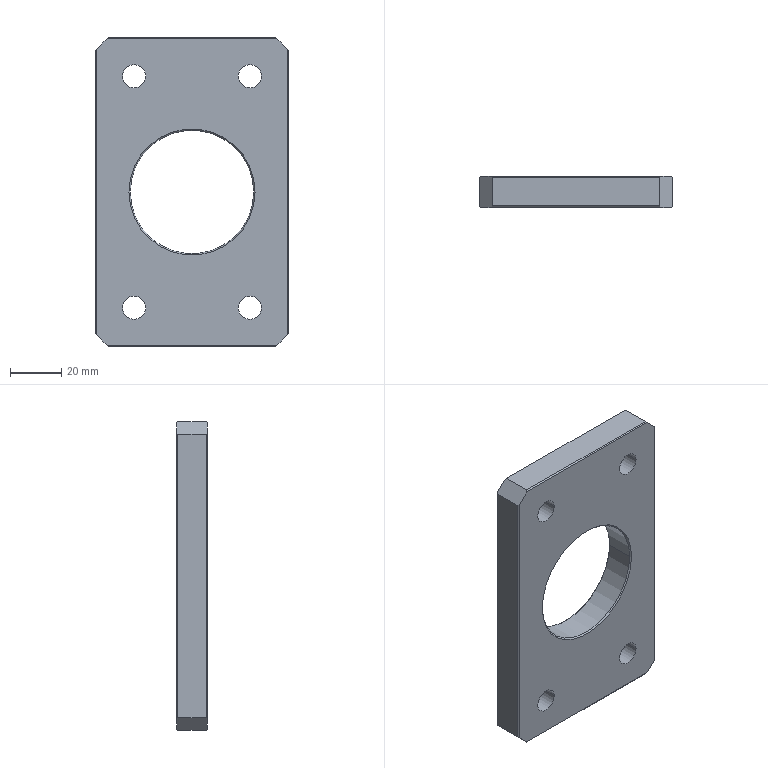Part | NX | 1 solid | 32 faces | box 75 x 12 x 120 mm | volume 82506 mm3 | plane 18 | cylinder 10 | cone 4 | commonest cylinder face diameters 9 x8 48 x2
STEP:
#1=CARTESIAN_POINT('',(-168.75,-112.,-577.5));
#2=VERTEX_POINT('',#1);
#3=CARTESIAN_POINT('',(-120.75,-112.,-577.5));
#4=VERTEX_POINT('',#3);
#5=CARTESIAN_POINT('',(-144.75,-112.,-577.5));
#6=DIRECTION('',(0.,-1.,0.));
#7=DIRECTION('',(0.,0.,-1.));
#8=AXIS2_PLACEMENT_3D('',#5,#6,#7);
#9=CIRCLE('',#8,24.);
#10=EDGE_CURVE('',#2,#4,#9,.T.);
#11=ORIENTED_EDGE('',*,*,#10,.T.);
#12=CARTESIAN_POINT('',(-120.75,-101.,-577.5));
#13=VERTEX_POINT('',#12);
#14=CARTESIAN_POINT('',(-120.75,-100.5,-577.5));
#15=DIRECTION('',(0.,1.,0.));
#16=VECTOR('',#15,1000.);
#17=LINE('',#14,#16);
#18=EDGE_CURVE('',#4,#13,#17,.T.);
#19=ORIENTED_EDGE('',*,*,#18,.T.);
#20=CARTESIAN_POINT('',(-168.75,-101.,-577.5));
#21=VERTEX_POINT('',#20);
#22=CARTESIAN_POINT('',(-144.75,-101.,-577.5));
#23=DIRECTION('',(0.,1.,0.));
#24=DIRECTION('',(0.,0.,1.));
#25=AXIS2_PLACEMENT_3D('',#22,#23,#24);
#26=CIRCLE('',#25,24.);
#27=EDGE_CURVE('',#13,#21,#26,.T.);
#28=ORIENTED_EDGE('',*,*,#27,.T.);
#29=CARTESIAN_POINT('',(-168.75,-100.5,-577.5));
#30=DIRECTION('',(0.,1.,0.));
#31=VECTOR('',#30,1000.);
#32=LINE('',#29,#31);
#33=EDGE_CURVE('',#2,#21,#32,.T.);
#34=ORIENTED_EDGE('',*,*,#33,.F.);
#35=EDGE_LOOP('',(#11,#19,#28,#34));
#36=FACE_BOUND('',#35,.T.);
#37=CARTESIAN_POINT('',(-144.75,-100.5,-577.5));
#38=DIRECTION('',(0.,1.,0.));
#39=DIRECTION('',(-1.,0.,0.));
#40=AXIS2_PLACEMENT_3D('',#37,#38,#39);
#41=CYLINDRICAL_SURFACE('',#40,24.);
#42=ADVANCED_FACE('',(#36),#41,.F.);
#43=CARTESIAN_POINT('',(-144.75,-101.,-577.5));
#44=DIRECTION('',(0.,1.,0.));
#45=DIRECTION('',(0.,0.,1.));
#46=AXIS2_PLACEMENT_3D('',#43,#44,#45);
#47=CIRCLE('',#46,24.);
#48=EDGE_CURVE('',#21,#13,#47,.T.);
#49=ORIENTED_EDGE('',*,*,#48,.F.);
#50=CARTESIAN_POINT('',(-169.25,-100.5,-577.5));
#51=VERTEX_POINT('',#50);
#52=CARTESIAN_POINT('',(-168.75,-101.,-577.5));
#53=DIRECTION('',(-0.7071,0.7071,0.));
#54=VECTOR('',#53,1000.);
#55=LINE('',#52,#54);
#56=EDGE_CURVE('',#51,#21,#55,.F.);
#57=ORIENTED_EDGE('',*,*,#56,.F.);
#58=CARTESIAN_POINT('',(-120.25,-100.5,-577.5));
#59=VERTEX_POINT('',#58);
#60=CARTESIAN_POINT('',(-144.75,-100.5,-577.5));
#61=DIRECTION('',(0.,1.,0.));
#62=DIRECTION('',(0.,0.,1.));
#63=AXIS2_PLACEMENT_3D('',#60,#61,#62);
#64=CIRCLE('',#63,24.5);
#65=EDGE_CURVE('',#51,#59,#64,.T.);
#66=ORIENTED_EDGE('',*,*,#65,.T.);
#67=CARTESIAN_POINT('',(-120.75,-101.,-577.5));
#68=DIRECTION('',(0.7071,0.7071,0.));
#69=VECTOR('',#68,1000.);
#70=LINE('',#67,#69);
#71=EDGE_CURVE('',#59,#13,#70,.F.);
#72=ORIENTED_EDGE('',*,*,#71,.T.);
#73=EDGE_LOOP('',(#49,#57,#66,#72));
#74=FACE_BOUND('',#73,.T.);
#75=CARTESIAN_POINT('',(-144.75,-101.,-577.5));
#76=DIRECTION('',(0.,1.,0.));
#77=DIRECTION('',(1.,0.,0.));
#78=AXIS2_PLACEMENT_3D('',#75,#76,#77);
#79=CONICAL_SURFACE('',#78,24.,0.7854);
#80=ADVANCED_FACE('',(#74),#79,.F.);
#81=CARTESIAN_POINT('',(-107.75,-100.5,-522.));
#82=VERTEX_POINT('',#81);
#83=CARTESIAN_POINT('',(-107.75,-100.5,-633.));
#84=VERTEX_POINT('',#83);
#85=CARTESIAN_POINT('',(-107.75,-100.5,-577.5));
#86=DIRECTION('',(0.,0.,-1.));
#87=VECTOR('',#86,1000.);
#88=LINE('',#85,#87);
#89=EDGE_CURVE('',#82,#84,#88,.T.);
#90=ORIENTED_EDGE('',*,*,#89,.T.);
#91=CARTESIAN_POINT('',(-111.75,-100.5,-637.));
#92=VERTEX_POINT('',#91);
#93=CARTESIAN_POINT('',(-11.5,-100.5,-536.75));
#94=DIRECTION('',(-0.7071,0.,-0.7071));
#95=VECTOR('',#94,1000.);
#96=LINE('',#93,#95);
#97=EDGE_CURVE('',#84,#92,#96,.T.);
#98=ORIENTED_EDGE('',*,*,#97,.T.);
#99=CARTESIAN_POINT('',(-177.75,-100.5,-637.));
#100=VERTEX_POINT('',#99);
#101=CARTESIAN_POINT('',(-11.5,-100.5,-637.));
#102=DIRECTION('',(-1.,0.,0.));
#103=VECTOR('',#102,1000.);
#104=LINE('',#101,#103);
#105=EDGE_CURVE('',#92,#100,#104,.T.);
#106=ORIENTED_EDGE('',*,*,#105,.T.);
#107=CARTESIAN_POINT('',(-181.75,-100.5,-633.));
#108=VERTEX_POINT('',#107);
#109=CARTESIAN_POINT('',(-11.5,-100.5,-803.25));
#110=DIRECTION('',(0.7071,0.,-0.7071));
#111=VECTOR('',#110,1000.);
#112=LINE('',#109,#111);
#113=EDGE_CURVE('',#108,#100,#112,.T.);
#114=ORIENTED_EDGE('',*,*,#113,.F.);
#115=CARTESIAN_POINT('',(-181.75,-100.5,-522.));
#116=VERTEX_POINT('',#115);
#117=CARTESIAN_POINT('',(-181.75,-100.5,-577.5));
#118=DIRECTION('',(0.,0.,1.));
#119=VECTOR('',#118,1000.);
#120=LINE('',#117,#119);
#121=EDGE_CURVE('',#108,#116,#120,.T.);
#122=ORIENTED_EDGE('',*,*,#121,.T.);
#123=CARTESIAN_POINT('',(-177.75,-100.5,-518.));
#124=VERTEX_POINT('',#123);
#125=CARTESIAN_POINT('',(-11.5,-100.5,-351.75));
#126=DIRECTION('',(-0.7071,0.,-0.7071));
#127=VECTOR('',#126,1000.);
#128=LINE('',#125,#127);
#129=EDGE_CURVE('',#124,#116,#128,.T.);
#130=ORIENTED_EDGE('',*,*,#129,.F.);
#131=CARTESIAN_POINT('',(-111.75,-100.5,-518.));
#132=VERTEX_POINT('',#131);
#133=CARTESIAN_POINT('',(-11.5,-100.5,-518.));
#134=DIRECTION('',(1.,0.,0.));
#135=VECTOR('',#134,1000.);
#136=LINE('',#133,#135);
#137=EDGE_CURVE('',#124,#132,#136,.T.);
#138=ORIENTED_EDGE('',*,*,#137,.T.);
#139=CARTESIAN_POINT('',(-11.5,-100.5,-618.25));
#140=DIRECTION('',(-0.7071,0.,0.7071));
#141=VECTOR('',#140,1000.);
#142=LINE('',#139,#141);
#143=EDGE_CURVE('',#82,#132,#142,.T.);
#144=ORIENTED_EDGE('',*,*,#143,.F.);
#145=EDGE_LOOP('',(#90,#98,#106,#114,#122,#130,#138,#144));
#146=FACE_BOUND('',#145,.T.);
#147=CARTESIAN_POINT('',(-126.75,-100.5,-622.5));
#148=VERTEX_POINT('',#147);
#149=CARTESIAN_POINT('',(-117.75,-100.5,-622.5));
#150=VERTEX_POINT('',#149);
#151=CARTESIAN_POINT('',(-122.25,-100.5,-622.5));
#152=DIRECTION('',(0.,1.,0.));
#153=DIRECTION('',(-1.,0.,0.));
#154=AXIS2_PLACEMENT_3D('',#151,#152,#153);
#155=CIRCLE('',#154,4.5);
#156=EDGE_CURVE('',#148,#150,#155,.T.);
#157=ORIENTED_EDGE('',*,*,#156,.F.);
#158=CARTESIAN_POINT('',(-122.25,-100.5,-622.5));
#159=DIRECTION('',(0.,1.,0.));
#160=DIRECTION('',(-1.,0.,0.));
#161=AXIS2_PLACEMENT_3D('',#158,#159,#160);
#162=CIRCLE('',#161,4.5);
#163=EDGE_CURVE('',#150,#148,#162,.T.);
#164=ORIENTED_EDGE('',*,*,#163,.F.);
#165=EDGE_LOOP('',(#157,#164));
#166=FACE_BOUND('',#165,.T.);
#167=CARTESIAN_POINT('',(-162.75,-100.5,-532.5));
#168=VERTEX_POINT('',#167);
#169=CARTESIAN_POINT('',(-171.75,-100.5,-532.5));
#170=VERTEX_POINT('',#169);
#171=CARTESIAN_POINT('',(-167.25,-100.5,-532.5));
#172=DIRECTION('',(0.,1.,0.));
#173=DIRECTION('',(-1.,0.,0.));
#174=AXIS2_PLACEMENT_3D('',#171,#172,#173);
#175=CIRCLE('',#174,4.5);
#176=EDGE_CURVE('',#168,#170,#175,.T.);
#177=ORIENTED_EDGE('',*,*,#176,.F.);
#178=CARTESIAN_POINT('',(-167.25,-100.5,-532.5));
#179=DIRECTION('',(0.,1.,0.));
#180=DIRECTION('',(-1.,0.,0.));
#181=AXIS2_PLACEMENT_3D('',#178,#179,#180);
#182=CIRCLE('',#181,4.5);
#183=EDGE_CURVE('',#170,#168,#182,.T.);
#184=ORIENTED_EDGE('',*,*,#183,.F.);
#185=EDGE_LOOP('',(#177,#184));
#186=FACE_BOUND('',#185,.T.);
#187=CARTESIAN_POINT('',(-126.75,-100.5,-532.5));
#188=VERTEX_POINT('',#187);
#189=CARTESIAN_POINT('',(-117.75,-100.5,-532.5));
#190=VERTEX_POINT('',#189);
#191=CARTESIAN_POINT('',(-122.25,-100.5,-532.5));
#192=DIRECTION('',(0.,1.,0.));
#193=DIRECTION('',(-1.,0.,0.));
#194=AXIS2_PLACEMENT_3D('',#191,#192,#193);
#195=CIRCLE('',#194,4.5);
#196=EDGE_CURVE('',#188,#190,#195,.T.);
#197=ORIENTED_EDGE('',*,*,#196,.F.);
#198=CARTESIAN_POINT('',(-122.25,-100.5,-532.5));
#199=DIRECTION('',(0.,1.,0.));
#200=DIRECTION('',(-1.,0.,0.));
#201=AXIS2_PLACEMENT_3D('',#198,#199,#200);
#202=CIRCLE('',#201,4.5);
#203=EDGE_CURVE('',#190,#188,#202,.T.);
#204=ORIENTED_EDGE('',*,*,#203,.F.);
#205=EDGE_LOOP('',(#197,#204));
#206=FACE_BOUND('',#205,.T.);
#207=CARTESIAN_POINT('',(-162.75,-100.5,-622.5));
#208=VERTEX_POINT('',#207);
#209=CARTESIAN_POINT('',(-171.75,-100.5,-622.5));
#210=VERTEX_POINT('',#209);
#211=CARTESIAN_POINT('',(-167.25,-100.5,-622.5));
#212=DIRECTION('',(0.,1.,0.));
#213=DIRECTION('',(-1.,0.,0.));
#214=AXIS2_PLACEMENT_3D('',#211,#212,#213);
#215=CIRCLE('',#214,4.5);
#216=EDGE_CURVE('',#208,#210,#215,.T.);
#217=ORIENTED_EDGE('',*,*,#216,.F.);
#218=CARTESIAN_POINT('',(-167.25,-100.5,-622.5));
#219=DIRECTION('',(0.,1.,0.));
#220=DIRECTION('',(-1.,0.,0.));
#221=AXIS2_PLACEMENT_3D('',#218,#219,#220);
#222=CIRCLE('',#221,4.5);
#223=EDGE_CURVE('',#210,#208,#222,.T.);
#224=ORIENTED_EDGE('',*,*,#223,.F.);
#225=EDGE_LOOP('',(#217,#224));
#226=FACE_BOUND('',#225,.T.);
#227=ORIENTED_EDGE('',*,*,#65,.F.);
#228=CARTESIAN_POINT('',(-144.75,-100.5,-577.5));
#229=DIRECTION('',(0.,1.,0.));
#230=DIRECTION('',(0.,0.,1.));
#231=AXIS2_PLACEMENT_3D('',#228,#229,#230);
#232=CIRCLE('',#231,24.5);
#233=EDGE_CURVE('',#59,#51,#232,.T.);
#234=ORIENTED_EDGE('',*,*,#233,.F.);
#235=EDGE_LOOP('',(#227,#234));
#236=FACE_BOUND('',#235,.T.);
#237=CARTESIAN_POINT('',(-38.847,-100.5,-601.077));
#238=DIRECTION('',(0.,1.,0.));
#239=DIRECTION('',(1.,0.,0.));
#240=AXIS2_PLACEMENT_3D('',#237,#238,#239);
#241=PLANE('',#240);
#242=ADVANCED_FACE('',(#146,#166,#186,#206,#226,#236),#241,.T.);
#243=ORIENTED_EDGE('',*,*,#89,.F.);
#244=CARTESIAN_POINT('',(-107.25,-101.,-522.5));
#245=VERTEX_POINT('',#244);
#246=CARTESIAN_POINT('',(-11.5,-196.75,-618.25));
#247=DIRECTION('',(-0.5774,0.5774,0.5774));
#248=VECTOR('',#247,1000.);
#249=LINE('',#246,#248);
#250=EDGE_CURVE('',#245,#82,#249,.T.);
#251=ORIENTED_EDGE('',*,*,#250,.F.);
#252=CARTESIAN_POINT('',(-107.25,-101.,-632.5));
#253=VERTEX_POINT('',#252);
#254=CARTESIAN_POINT('',(-107.25,-101.,-577.5));
#255=DIRECTION('',(0.,0.,1.));
#256=VECTOR('',#255,1000.);
#257=LINE('',#254,#256);
#258=EDGE_CURVE('',#253,#245,#257,.T.);
#259=ORIENTED_EDGE('',*,*,#258,.F.);
#260=CARTESIAN_POINT('',(-11.5,-196.75,-536.75));
#261=DIRECTION('',(-0.5774,0.5774,-0.5774));
#262=VECTOR('',#261,1000.);
#263=LINE('',#260,#262);
#264=EDGE_CURVE('',#253,#84,#263,.T.);
#265=ORIENTED_EDGE('',*,*,#264,.T.);
#266=EDGE_LOOP('',(#243,#251,#259,#265));
#267=FACE_BOUND('',#266,.T.);
#268=CARTESIAN_POINT('',(-107.5,-100.75,-577.5));
#269=DIRECTION('',(-0.7071,-0.7071,0.));
#270=DIRECTION('',(-0.7071,0.7071,0.));
#271=AXIS2_PLACEMENT_3D('',#268,#269,#270);
#272=PLANE('',#271);
#273=ADVANCED_FACE('',(#267),#272,.F.);
#274=CARTESIAN_POINT('',(-107.25,-112.,-632.5));
#275=VERTEX_POINT('',#274);
#276=CARTESIAN_POINT('',(-107.25,-106.5,-632.5));
#277=DIRECTION('',(0.,1.,0.));
#278=VECTOR('',#277,1000.);
#279=LINE('',#276,#278);
#280=EDGE_CURVE('',#275,#253,#279,.T.);
#281=ORIENTED_EDGE('',*,*,#280,.T.);
#282=ORIENTED_EDGE('',*,*,#258,.T.);
#283=CARTESIAN_POINT('',(-107.25,-112.,-522.5));
#284=VERTEX_POINT('',#283);
#285=CARTESIAN_POINT('',(-107.25,-106.5,-522.5));
#286=DIRECTION('',(0.,1.,0.));
#287=VECTOR('',#286,1000.);
#288=LINE('',#285,#287);
#289=EDGE_CURVE('',#284,#245,#288,.T.);
#290=ORIENTED_EDGE('',*,*,#289,.F.);
#291=CARTESIAN_POINT('',(-107.25,-112.,-577.5));
#292=DIRECTION('',(0.,0.,1.));
#293=VECTOR('',#292,1000.);
#294=LINE('',#291,#293);
#295=EDGE_CURVE('',#275,#284,#294,.T.);
#296=ORIENTED_EDGE('',*,*,#295,.F.);
#297=EDGE_LOOP('',(#281,#282,#290,#296));
#298=FACE_BOUND('',#297,.T.);
#299=CARTESIAN_POINT('',(-107.25,-100.5,-517.5));
#300=DIRECTION('',(1.,0.,0.));
#301=DIRECTION('',(0.,1.,0.));
#302=AXIS2_PLACEMENT_3D('',#299,#300,#301);
#303=PLANE('',#302);
#304=ADVANCED_FACE('',(#298),#303,.T.);
#305=CARTESIAN_POINT('',(-177.25,-112.,-517.5));
#306=VERTEX_POINT('',#305);
#307=CARTESIAN_POINT('',(-177.25,-101.,-517.5));
#308=VERTEX_POINT('',#307);
#309=CARTESIAN_POINT('',(-177.25,-106.5,-517.5));
#310=DIRECTION('',(0.,1.,0.));
#311=VECTOR('',#310,1000.);
#312=LINE('',#309,#311);
#313=EDGE_CURVE('',#306,#308,#312,.T.);
#314=ORIENTED_EDGE('',*,*,#313,.F.);
#315=CARTESIAN_POINT('',(-112.25,-112.,-517.5));
#316=VERTEX_POINT('',#315);
#317=CARTESIAN_POINT('',(-11.5,-112.,-517.5));
#318=DIRECTION('',(-1.,0.,0.));
#319=VECTOR('',#318,1000.);
#320=LINE('',#317,#319);
#321=EDGE_CURVE('',#316,#306,#320,.T.);
#322=ORIENTED_EDGE('',*,*,#321,.F.);
#323=CARTESIAN_POINT('',(-112.25,-101.,-517.5));
#324=VERTEX_POINT('',#323);
#325=CARTESIAN_POINT('',(-112.25,-106.5,-517.5));
#326=DIRECTION('',(0.,-1.,0.));
#327=VECTOR('',#326,1000.);
#328=LINE('',#325,#327);
#329=EDGE_CURVE('',#324,#316,#328,.T.);
#330=ORIENTED_EDGE('',*,*,#329,.F.);
#331=CARTESIAN_POINT('',(-11.5,-101.,-517.5));
#332=DIRECTION('',(-1.,0.,0.));
#333=VECTOR('',#332,1000.);
#334=LINE('',#331,#333);
#335=EDGE_CURVE('',#324,#308,#334,.T.);
#336=ORIENTED_EDGE('',*,*,#335,.T.);
#337=EDGE_LOOP('',(#314,#322,#330,#336));
#338=FACE_BOUND('',#337,.T.);
#339=CARTESIAN_POINT('',(-182.25,-100.5,-517.5));
#340=DIRECTION('',(0.,0.,1.));
#341=DIRECTION('',(1.,0.,0.));
#342=AXIS2_PLACEMENT_3D('',#339,#340,#341);
#343=PLANE('',#342);
#344=ADVANCED_FACE('',(#338),#343,.T.);
#345=CARTESIAN_POINT('',(-182.25,-112.,-632.5));
#346=VERTEX_POINT('',#345);
#347=CARTESIAN_POINT('',(-182.25,-101.,-632.5));
#348=VERTEX_POINT('',#347);
#349=CARTESIAN_POINT('',(-182.25,-106.5,-632.5));
#350=DIRECTION('',(0.,1.,0.));
#351=VECTOR('',#350,1000.);
#352=LINE('',#349,#351);
#353=EDGE_CURVE('',#346,#348,#352,.T.);
#354=ORIENTED_EDGE('',*,*,#353,.F.);
#355=CARTESIAN_POINT('',(-182.25,-112.,-522.5));
#356=VERTEX_POINT('',#355);
#357=CARTESIAN_POINT('',(-182.25,-112.,-577.5));
#358=DIRECTION('',(0.,0.,-1.));
#359=VECTOR('',#358,1000.);
#360=LINE('',#357,#359);
#361=EDGE_CURVE('',#356,#346,#360,.T.);
#362=ORIENTED_EDGE('',*,*,#361,.F.);
#363=CARTESIAN_POINT('',(-182.25,-101.,-522.5));
#364=VERTEX_POINT('',#363);
#365=CARTESIAN_POINT('',(-182.25,-106.5,-522.5));
#366=DIRECTION('',(0.,-1.,0.));
#367=VECTOR('',#366,1000.);
#368=LINE('',#365,#367);
#369=EDGE_CURVE('',#364,#356,#368,.T.);
#370=ORIENTED_EDGE('',*,*,#369,.F.);
#371=CARTESIAN_POINT('',(-182.25,-101.,-577.5));
#372=DIRECTION('',(0.,0.,-1.));
#373=VECTOR('',#372,1000.);
#374=LINE('',#371,#373);
#375=EDGE_CURVE('',#364,#348,#374,.T.);
#376=ORIENTED_EDGE('',*,*,#375,.T.);
#377=EDGE_LOOP('',(#354,#362,#370,#376));
#378=FACE_BOUND('',#377,.T.);
#379=CARTESIAN_POINT('',(-182.25,-100.5,-637.5));
#380=DIRECTION('',(-1.,0.,0.));
#381=DIRECTION('',(0.,0.,1.));
#382=AXIS2_PLACEMENT_3D('',#379,#380,#381);
#383=PLANE('',#382);
#384=ADVANCED_FACE('',(#378),#383,.T.);
#385=CARTESIAN_POINT('',(-177.25,-101.,-637.5));
#386=VERTEX_POINT('',#385);
#387=CARTESIAN_POINT('',(-112.25,-101.,-637.5));
#388=VERTEX_POINT('',#387);
#389=CARTESIAN_POINT('',(-11.5,-101.,-637.5));
#390=DIRECTION('',(1.,0.,0.));
#391=VECTOR('',#390,1000.);
#392=LINE('',#389,#391);
#393=EDGE_CURVE('',#386,#388,#392,.T.);
#394=ORIENTED_EDGE('',*,*,#393,.T.);
#395=CARTESIAN_POINT('',(-112.25,-112.,-637.5));
#396=VERTEX_POINT('',#395);
#397=CARTESIAN_POINT('',(-112.25,-106.5,-637.5));
#398=DIRECTION('',(0.,-1.,0.));
#399=VECTOR('',#398,1000.);
#400=LINE('',#397,#399);
#401=EDGE_CURVE('',#388,#396,#400,.T.);
#402=ORIENTED_EDGE('',*,*,#401,.T.);
#403=CARTESIAN_POINT('',(-177.25,-112.,-637.5));
#404=VERTEX_POINT('',#403);
#405=CARTESIAN_POINT('',(-11.5,-112.,-637.5));
#406=DIRECTION('',(1.,0.,0.));
#407=VECTOR('',#406,1000.);
#408=LINE('',#405,#407);
#409=EDGE_CURVE('',#404,#396,#408,.T.);
#410=ORIENTED_EDGE('',*,*,#409,.F.);
#411=CARTESIAN_POINT('',(-177.25,-106.5,-637.5));
#412=DIRECTION('',(0.,-1.,0.));
#413=VECTOR('',#412,1000.);
#414=LINE('',#411,#413);
#415=EDGE_CURVE('',#386,#404,#414,.T.);
#416=ORIENTED_EDGE('',*,*,#415,.F.);
#417=EDGE_LOOP('',(#394,#402,#410,#416));
#418=FACE_BOUND('',#417,.T.);
#419=CARTESIAN_POINT('',(-107.25,-100.5,-637.5));
#420=DIRECTION('',(0.,0.,-1.));
#421=DIRECTION('',(0.,-1.,0.));
#422=AXIS2_PLACEMENT_3D('',#419,#420,#421);
#423=PLANE('',#422);
#424=ADVANCED_FACE('',(#418),#423,.T.);
#425=ORIENTED_EDGE('',*,*,#313,.T.);
#426=CARTESIAN_POINT('',(-11.5,-266.75,-351.75));
#427=DIRECTION('',(-0.5774,0.5774,-0.5774));
#428=VECTOR('',#427,1000.);
#429=LINE('',#426,#428);
#430=EDGE_CURVE('',#308,#124,#429,.T.);
#431=ORIENTED_EDGE('',*,*,#430,.T.);
#432=ORIENTED_EDGE('',*,*,#129,.T.);
#433=CARTESIAN_POINT('',(-11.5,69.75,-351.75));
#434=DIRECTION('',(-0.5774,-0.5774,-0.5774));
#435=VECTOR('',#434,1000.);
#436=LINE('',#433,#435);
#437=EDGE_CURVE('',#116,#364,#436,.T.);
#438=ORIENTED_EDGE('',*,*,#437,.T.);
#439=ORIENTED_EDGE('',*,*,#369,.T.);
#440=CARTESIAN_POINT('',(-181.75,-112.5,-522.));
#441=VERTEX_POINT('',#440);
#442=CARTESIAN_POINT('',(-11.5,-282.75,-351.75));
#443=DIRECTION('',(-0.5774,0.5774,-0.5774));
#444=VECTOR('',#443,1000.);
#445=LINE('',#442,#444);
#446=EDGE_CURVE('',#441,#356,#445,.T.);
#447=ORIENTED_EDGE('',*,*,#446,.F.);
#448=CARTESIAN_POINT('',(-177.75,-112.5,-518.));
#449=VERTEX_POINT('',#448);
#450=CARTESIAN_POINT('',(-11.5,-112.5,-351.75));
#451=DIRECTION('',(-0.7071,0.,-0.7071));
#452=VECTOR('',#451,1000.);
#453=LINE('',#450,#452);
#454=EDGE_CURVE('',#449,#441,#453,.T.);
#455=ORIENTED_EDGE('',*,*,#454,.F.);
#456=CARTESIAN_POINT('',(-11.5,53.75,-351.75));
#457=DIRECTION('',(-0.5774,-0.5774,-0.5774));
#458=VECTOR('',#457,1000.);
#459=LINE('',#456,#458);
#460=EDGE_CURVE('',#306,#449,#459,.T.);
#461=ORIENTED_EDGE('',*,*,#460,.F.);
#462=EDGE_LOOP('',(#425,#431,#432,#438,#439,#447,#455,#461));
#463=FACE_BOUND('',#462,.T.);
#464=CARTESIAN_POINT('',(-179.75,-106.5,-520.));
#465=DIRECTION('',(-0.7071,0.,0.7071));
#466=DIRECTION('',(0.,1.,0.));
#467=AXIS2_PLACEMENT_3D('',#464,#465,#466);
#468=PLANE('',#467);
#469=ADVANCED_FACE('',(#463),#468,.T.);
#470=ORIENTED_EDGE('',*,*,#353,.T.);
#471=CARTESIAN_POINT('',(-11.5,69.75,-803.25));
#472=DIRECTION('',(0.5774,0.5774,-0.5774));
#473=VECTOR('',#472,1000.);
#474=LINE('',#471,#473);
#475=EDGE_CURVE('',#348,#108,#474,.T.);
#476=ORIENTED_EDGE('',*,*,#475,.T.);
#477=ORIENTED_EDGE('',*,*,#113,.T.);
#478=CARTESIAN_POINT('',(-11.5,-266.75,-803.25));
#479=DIRECTION('',(0.5774,-0.5774,-0.5774));
#480=VECTOR('',#479,1000.);
#481=LINE('',#478,#480);
#482=EDGE_CURVE('',#100,#386,#481,.T.);
#483=ORIENTED_EDGE('',*,*,#482,.T.);
#484=ORIENTED_EDGE('',*,*,#415,.T.);
#485=CARTESIAN_POINT('',(-177.75,-112.5,-637.));
#486=VERTEX_POINT('',#485);
#487=CARTESIAN_POINT('',(-11.5,53.75,-803.25));
#488=DIRECTION('',(0.5774,0.5774,-0.5774));
#489=VECTOR('',#488,1000.);
#490=LINE('',#487,#489);
#491=EDGE_CURVE('',#486,#404,#490,.T.);
#492=ORIENTED_EDGE('',*,*,#491,.F.);
#493=CARTESIAN_POINT('',(-181.75,-112.5,-633.));
#494=VERTEX_POINT('',#493);
#495=CARTESIAN_POINT('',(-11.5,-112.5,-803.25));
#496=DIRECTION('',(0.7071,0.,-0.7071));
#497=VECTOR('',#496,1000.);
#498=LINE('',#495,#497);
#499=EDGE_CURVE('',#494,#486,#498,.T.);
#500=ORIENTED_EDGE('',*,*,#499,.F.);
#501=CARTESIAN_POINT('',(-11.5,-282.75,-803.25));
#502=DIRECTION('',(0.5774,-0.5774,-0.5774));
#503=VECTOR('',#502,1000.);
#504=LINE('',#501,#503);
#505=EDGE_CURVE('',#346,#494,#504,.T.);
#506=ORIENTED_EDGE('',*,*,#505,.F.);
#507=EDGE_LOOP('',(#470,#476,#477,#483,#484,#492,#500,#506));
#508=FACE_BOUND('',#507,.T.);
#509=CARTESIAN_POINT('',(-179.75,-106.5,-635.));
#510=DIRECTION('',(-0.7071,0.,-0.7071));
#511=DIRECTION('',(-0.7071,0.,0.7071));
#512=AXIS2_PLACEMENT_3D('',#509,#510,#511);
#513=PLANE('',#512);
#514=ADVANCED_FACE('',(#508),#513,.T.);
#515=ORIENTED_EDGE('',*,*,#289,.T.);
#516=ORIENTED_EDGE('',*,*,#250,.T.);
#517=ORIENTED_EDGE('',*,*,#143,.T.);
#518=CARTESIAN_POINT('',(-11.5,-0.25,-618.25));
#519=DIRECTION('',(-0.5774,-0.5774,0.5774));
#520=VECTOR('',#519,1000.);
#521=LINE('',#518,#520);
#522=EDGE_CURVE('',#132,#324,#521,.T.);
#523=ORIENTED_EDGE('',*,*,#522,.T.);
#524=ORIENTED_EDGE('',*,*,#329,.T.);
#525=CARTESIAN_POINT('',(-111.75,-112.5,-518.));
#526=VERTEX_POINT('',#525);
#527=CARTESIAN_POINT('',(-11.5,-212.75,-618.25));
#528=DIRECTION('',(-0.5774,0.5774,0.5774));
#529=VECTOR('',#528,1000.);
#530=LINE('',#527,#529);
#531=EDGE_CURVE('',#526,#316,#530,.T.);
#532=ORIENTED_EDGE('',*,*,#531,.F.);
#533=CARTESIAN_POINT('',(-107.75,-112.5,-522.));
#534=VERTEX_POINT('',#533);
#535=CARTESIAN_POINT('',(-11.5,-112.5,-618.25));
#536=DIRECTION('',(-0.7071,0.,0.7071));
#537=VECTOR('',#536,1000.);
#538=LINE('',#535,#537);
#539=EDGE_CURVE('',#534,#526,#538,.T.);
#540=ORIENTED_EDGE('',*,*,#539,.F.);
#541=CARTESIAN_POINT('',(-11.5,-16.25,-618.25));
#542=DIRECTION('',(-0.5774,-0.5774,0.5774));
#543=VECTOR('',#542,1000.);
#544=LINE('',#541,#543);
#545=EDGE_CURVE('',#284,#534,#544,.T.);
#546=ORIENTED_EDGE('',*,*,#545,.F.);
#547=EDGE_LOOP('',(#515,#516,#517,#523,#524,#532,#540,#546));
#548=FACE_BOUND('',#547,.T.);
#549=CARTESIAN_POINT('',(-109.75,-106.5,-520.));
#550=DIRECTION('',(0.7071,0.,0.7071));
#551=DIRECTION('',(0.,-1.,0.));
#552=AXIS2_PLACEMENT_3D('',#549,#550,#551);
#553=PLANE('',#552);
#554=ADVANCED_FACE('',(#548),#553,.T.);
#555=ORIENTED_EDGE('',*,*,#280,.F.);
#556=CARTESIAN_POINT('',(-107.75,-112.5,-633.));
#557=VERTEX_POINT('',#556);
#558=CARTESIAN_POINT('',(-11.5,-16.25,-536.75));
#559=DIRECTION('',(-0.5774,-0.5774,-0.5774));
#560=VECTOR('',#559,1000.);
#561=LINE('',#558,#560);
#562=EDGE_CURVE('',#275,#557,#561,.T.);
#563=ORIENTED_EDGE('',*,*,#562,.T.);
#564=CARTESIAN_POINT('',(-111.75,-112.5,-637.));
#565=VERTEX_POINT('',#564);
#566=CARTESIAN_POINT('',(-11.5,-112.5,-536.75));
#567=DIRECTION('',(-0.7071,0.,-0.7071));
#568=VECTOR('',#567,1000.);
#569=LINE('',#566,#568);
#570=EDGE_CURVE('',#557,#565,#569,.T.);
#571=ORIENTED_EDGE('',*,*,#570,.T.);
#572=CARTESIAN_POINT('',(-11.5,-212.75,-536.75));
#573=DIRECTION('',(-0.5774,0.5774,-0.5774));
#574=VECTOR('',#573,1000.);
#575=LINE('',#572,#574);
#576=EDGE_CURVE('',#565,#396,#575,.T.);
#577=ORIENTED_EDGE('',*,*,#576,.T.);
#578=ORIENTED_EDGE('',*,*,#401,.F.);
#579=CARTESIAN_POINT('',(-11.5,-0.25,-536.75));
#580=DIRECTION('',(-0.5774,-0.5774,-0.5774));
#581=VECTOR('',#580,1000.);
#582=LINE('',#579,#581);
#583=EDGE_CURVE('',#92,#388,#582,.T.);
#584=ORIENTED_EDGE('',*,*,#583,.F.);
#585=ORIENTED_EDGE('',*,*,#97,.F.);
#586=ORIENTED_EDGE('',*,*,#264,.F.);
#587=EDGE_LOOP('',(#555,#563,#571,#577,#578,#584,#585,#586));
#588=FACE_BOUND('',#587,.T.);
#589=CARTESIAN_POINT('',(-109.75,-106.5,-635.));
#590=DIRECTION('',(-0.7071,0.,0.7071));
#591=DIRECTION('',(0.,1.,0.));
#592=AXIS2_PLACEMENT_3D('',#589,#590,#591);
#593=PLANE('',#592);
#594=ADVANCED_FACE('',(#588),#593,.F.);
#595=CARTESIAN_POINT('',(-171.75,-112.5,-532.5));
#596=VERTEX_POINT('',#595);
#597=CARTESIAN_POINT('',(-162.75,-112.5,-532.5));
#598=VERTEX_POINT('',#597);
#599=CARTESIAN_POINT('',(-167.25,-112.5,-532.5));
#600=DIRECTION('',(0.,1.,0.));
#601=DIRECTION('',(-1.,0.,0.));
#602=AXIS2_PLACEMENT_3D('',#599,#600,#601);
#603=CIRCLE('',#602,4.5);
#604=EDGE_CURVE('',#596,#598,#603,.T.);
#605=ORIENTED_EDGE('',*,*,#604,.F.);
#606=CARTESIAN_POINT('',(-171.75,-100.5,-532.5));
#607=DIRECTION('',(0.,1.,0.));
#608=VECTOR('',#607,1000.);
#609=LINE('',#606,#608);
#610=EDGE_CURVE('',#170,#596,#609,.F.);
#611=ORIENTED_EDGE('',*,*,#610,.F.);
#612=ORIENTED_EDGE('',*,*,#183,.T.);
#613=CARTESIAN_POINT('',(-162.75,-100.5,-532.5));
#614=DIRECTION('',(0.,1.,0.));
#615=VECTOR('',#614,1000.);
#616=LINE('',#613,#615);
#617=EDGE_CURVE('',#168,#598,#616,.F.);
#618=ORIENTED_EDGE('',*,*,#617,.T.);
#619=EDGE_LOOP('',(#605,#611,#612,#618));
#620=FACE_BOUND('',#619,.T.);
#621=CARTESIAN_POINT('',(-167.25,-100.5,-532.5));
#622=DIRECTION('',(0.,1.,0.));
#623=DIRECTION('',(-1.,0.,0.));
#624=AXIS2_PLACEMENT_3D('',#621,#622,#623);
#625=CYLINDRICAL_SURFACE('',#624,4.5);
#626=ADVANCED_FACE('',(#620),#625,.F.);
#627=ORIENTED_EDGE('',*,*,#105,.F.);
#628=ORIENTED_EDGE('',*,*,#583,.T.);
#629=ORIENTED_EDGE('',*,*,#393,.F.);
#630=ORIENTED_EDGE('',*,*,#482,.F.);
#631=EDGE_LOOP('',(#627,#628,#629,#630));
#632=FACE_BOUND('',#631,.T.);
#633=CARTESIAN_POINT('',(-144.75,-100.75,-637.25));
#634=DIRECTION('',(0.,-0.7071,0.7071));
#635=DIRECTION('',(-1.,0.,0.));
#636=AXIS2_PLACEMENT_3D('',#633,#634,#635);
#637=PLANE('',#636);
#638=ADVANCED_FACE('',(#632),#637,.F.);
#639=ORIENTED_EDGE('',*,*,#156,.T.);
#640=CARTESIAN_POINT('',(-117.75,-112.5,-622.5));
#641=VERTEX_POINT('',#640);
#642=CARTESIAN_POINT('',(-117.75,-100.5,-622.5));
#643=DIRECTION('',(0.,1.,0.));
#644=VECTOR('',#643,1000.);
#645=LINE('',#642,#644);
#646=EDGE_CURVE('',#150,#641,#645,.F.);
#647=ORIENTED_EDGE('',*,*,#646,.T.);
#648=CARTESIAN_POINT('',(-126.75,-112.5,-622.5));
#649=VERTEX_POINT('',#648);
#650=CARTESIAN_POINT('',(-122.25,-112.5,-622.5));
#651=DIRECTION('',(0.,1.,0.));
#652=DIRECTION('',(-1.,0.,0.));
#653=AXIS2_PLACEMENT_3D('',#650,#651,#652);
#654=CIRCLE('',#653,4.5);
#655=EDGE_CURVE('',#649,#641,#654,.T.);
#656=ORIENTED_EDGE('',*,*,#655,.F.);
#657=CARTESIAN_POINT('',(-126.75,-100.5,-622.5));
#658=DIRECTION('',(0.,1.,0.));
#659=VECTOR('',#658,1000.);
#660=LINE('',#657,#659);
#661=EDGE_CURVE('',#148,#649,#660,.F.);
#662=ORIENTED_EDGE('',*,*,#661,.F.);
#663=EDGE_LOOP('',(#639,#647,#656,#662));
#664=FACE_BOUND('',#663,.T.);
#665=CARTESIAN_POINT('',(-122.25,-100.5,-622.5));
#666=DIRECTION('',(0.,1.,0.));
#667=DIRECTION('',(-1.,0.,0.));
#668=AXIS2_PLACEMENT_3D('',#665,#666,#667);
#669=CYLINDRICAL_SURFACE('',#668,4.5);
#670=ADVANCED_FACE('',(#664),#669,.F.);
#671=CARTESIAN_POINT('',(-120.25,-112.5,-577.5));
#672=VERTEX_POINT('',#671);
#673=CARTESIAN_POINT('',(-169.25,-112.5,-577.5));
#674=VERTEX_POINT('',#673);
#675=CARTESIAN_POINT('',(-144.75,-112.5,-577.5));
#676=DIRECTION('',(0.,-1.,0.));
#677=DIRECTION('',(0.,0.,-1.));
#678=AXIS2_PLACEMENT_3D('',#675,#676,#677);
#679=CIRCLE('',#678,24.5);
#680=EDGE_CURVE('',#672,#674,#679,.T.);
#681=ORIENTED_EDGE('',*,*,#680,.T.);
#682=CARTESIAN_POINT('',(-169.25,-112.5,-577.5));
#683=DIRECTION('',(-0.7071,-0.7071,0.));
#684=VECTOR('',#683,1000.);
#685=LINE('',#682,#684);
#686=EDGE_CURVE('',#674,#2,#685,.F.);
#687=ORIENTED_EDGE('',*,*,#686,.T.);
#688=CARTESIAN_POINT('',(-144.75,-112.,-577.5));
#689=DIRECTION('',(0.,-1.,0.));
#690=DIRECTION('',(0.,0.,-1.));
#691=AXIS2_PLACEMENT_3D('',#688,#689,#690);
#692=CIRCLE('',#691,24.);
#693=EDGE_CURVE('',#4,#2,#692,.T.);
#694=ORIENTED_EDGE('',*,*,#693,.F.);
#695=CARTESIAN_POINT('',(-120.25,-112.5,-577.5));
#696=DIRECTION('',(0.7071,-0.7071,0.));
#697=VECTOR('',#696,1000.);
#698=LINE('',#695,#697);
#699=EDGE_CURVE('',#672,#4,#698,.F.);
#700=ORIENTED_EDGE('',*,*,#699,.F.);
#701=EDGE_LOOP('',(#681,#687,#694,#700));
#702=FACE_BOUND('',#701,.T.);
#703=CARTESIAN_POINT('',(-144.75,-112.5,-577.5));
#704=DIRECTION('',(0.,-1.,0.));
#705=DIRECTION('',(-1.,0.,0.));
#706=AXIS2_PLACEMENT_3D('',#703,#704,#705);
#707=CONICAL_SURFACE('',#706,24.5,0.7854);
#708=ADVANCED_FACE('',(#702),#707,.F.);
#709=ORIENTED_EDGE('',*,*,#196,.T.);
#710=CARTESIAN_POINT('',(-117.75,-112.5,-532.5));
#711=VERTEX_POINT('',#710);
#712=CARTESIAN_POINT('',(-117.75,-100.5,-532.5));
#713=DIRECTION('',(0.,1.,0.));
#714=VECTOR('',#713,1000.);
#715=LINE('',#712,#714);
#716=EDGE_CURVE('',#190,#711,#715,.F.);
#717=ORIENTED_EDGE('',*,*,#716,.T.);
#718=CARTESIAN_POINT('',(-126.75,-112.5,-532.5));
#719=VERTEX_POINT('',#718);
#720=CARTESIAN_POINT('',(-122.25,-112.5,-532.5));
#721=DIRECTION('',(0.,1.,0.));
#722=DIRECTION('',(-1.,0.,0.));
#723=AXIS2_PLACEMENT_3D('',#720,#721,#722);
#724=CIRCLE('',#723,4.5);
#725=EDGE_CURVE('',#719,#711,#724,.T.);
#726=ORIENTED_EDGE('',*,*,#725,.F.);
#727=CARTESIAN_POINT('',(-126.75,-100.5,-532.5));
#728=DIRECTION('',(0.,1.,0.));
#729=VECTOR('',#728,1000.);
#730=LINE('',#727,#729);
#731=EDGE_CURVE('',#188,#719,#730,.F.);
#732=ORIENTED_EDGE('',*,*,#731,.F.);
#733=EDGE_LOOP('',(#709,#717,#726,#732));
#734=FACE_BOUND('',#733,.T.);
#735=CARTESIAN_POINT('',(-122.25,-100.5,-532.5));
#736=DIRECTION('',(0.,1.,0.));
#737=DIRECTION('',(-1.,0.,0.));
#738=AXIS2_PLACEMENT_3D('',#735,#736,#737);
#739=CYLINDRICAL_SURFACE('',#738,4.5);
#740=ADVANCED_FACE('',(#734),#739,.F.);
#741=ORIENTED_EDGE('',*,*,#137,.F.);
#742=ORIENTED_EDGE('',*,*,#430,.F.);
#743=ORIENTED_EDGE('',*,*,#335,.F.);
#744=ORIENTED_EDGE('',*,*,#522,.F.);
#745=EDGE_LOOP('',(#741,#742,#743,#744));
#746=FACE_BOUND('',#745,.T.);
#747=CARTESIAN_POINT('',(-144.75,-100.75,-517.75));
#748=DIRECTION('',(0.,-0.7071,-0.7071));
#749=DIRECTION('',(0.,-0.7071,0.7071));
#750=AXIS2_PLACEMENT_3D('',#747,#748,#749);
#751=PLANE('',#750);
#752=ADVANCED_FACE('',(#746),#751,.F.);
#753=CARTESIAN_POINT('',(-162.75,-112.5,-622.5));
#754=VERTEX_POINT('',#753);
#755=CARTESIAN_POINT('',(-171.75,-112.5,-622.5));
#756=VERTEX_POINT('',#755);
#757=CARTESIAN_POINT('',(-167.25,-112.5,-622.5));
#758=DIRECTION('',(0.,1.,0.));
#759=DIRECTION('',(-1.,0.,0.));
#760=AXIS2_PLACEMENT_3D('',#757,#758,#759);
#761=CIRCLE('',#760,4.5);
#762=EDGE_CURVE('',#754,#756,#761,.T.);
#763=ORIENTED_EDGE('',*,*,#762,.F.);
#764=CARTESIAN_POINT('',(-162.75,-100.5,-622.5));
#765=DIRECTION('',(0.,1.,0.));
#766=VECTOR('',#765,1000.);
#767=LINE('',#764,#766);
#768=EDGE_CURVE('',#208,#754,#767,.F.);
#769=ORIENTED_EDGE('',*,*,#768,.F.);
#770=ORIENTED_EDGE('',*,*,#216,.T.);
#771=CARTESIAN_POINT('',(-171.75,-100.5,-622.5));
#772=DIRECTION('',(0.,1.,0.));
#773=VECTOR('',#772,1000.);
#774=LINE('',#771,#773);
#775=EDGE_CURVE('',#210,#756,#774,.F.);
#776=ORIENTED_EDGE('',*,*,#775,.T.);
#777=EDGE_LOOP('',(#763,#769,#770,#776));
#778=FACE_BOUND('',#777,.T.);
#779=CARTESIAN_POINT('',(-167.25,-100.5,-622.5));
#780=DIRECTION('',(0.,1.,0.));
#781=DIRECTION('',(-1.,0.,0.));
#782=AXIS2_PLACEMENT_3D('',#779,#780,#781);
#783=CYLINDRICAL_SURFACE('',#782,4.5);
#784=ADVANCED_FACE('',(#778),#783,.F.);
#785=ORIENTED_EDGE('',*,*,#121,.F.);
#786=ORIENTED_EDGE('',*,*,#475,.F.);
#787=ORIENTED_EDGE('',*,*,#375,.F.);
#788=ORIENTED_EDGE('',*,*,#437,.F.);
#789=EDGE_LOOP('',(#785,#786,#787,#788));
#790=FACE_BOUND('',#789,.T.);
#791=CARTESIAN_POINT('',(-182.,-100.75,-577.5));
#792=DIRECTION('',(0.7071,-0.7071,0.));
#793=DIRECTION('',(0.,0.,-1.));
#794=AXIS2_PLACEMENT_3D('',#791,#792,#793);
#795=PLANE('',#794);
#796=ADVANCED_FACE('',(#790),#795,.F.);
#797=CARTESIAN_POINT('',(-11.5,-112.5,-637.));
#798=DIRECTION('',(1.,0.,0.));
#799=VECTOR('',#798,1000.);
#800=LINE('',#797,#799);
#801=EDGE_CURVE('',#486,#565,#800,.T.);
#802=ORIENTED_EDGE('',*,*,#801,.T.);
#803=ORIENTED_EDGE('',*,*,#570,.F.);
#804=CARTESIAN_POINT('',(-107.75,-112.5,-577.5));
#805=DIRECTION('',(0.,0.,1.));
#806=VECTOR('',#805,1000.);
#807=LINE('',#804,#806);
#808=EDGE_CURVE('',#557,#534,#807,.T.);
#809=ORIENTED_EDGE('',*,*,#808,.T.);
#810=ORIENTED_EDGE('',*,*,#539,.T.);
#811=CARTESIAN_POINT('',(-11.5,-112.5,-518.));
#812=DIRECTION('',(-1.,0.,0.));
#813=VECTOR('',#812,1000.);
#814=LINE('',#811,#813);
#815=EDGE_CURVE('',#526,#449,#814,.T.);
#816=ORIENTED_EDGE('',*,*,#815,.T.);
#817=ORIENTED_EDGE('',*,*,#454,.T.);
#818=CARTESIAN_POINT('',(-181.75,-112.5,-577.5));
#819=DIRECTION('',(0.,0.,-1.));
#820=VECTOR('',#819,1000.);
#821=LINE('',#818,#820);
#822=EDGE_CURVE('',#441,#494,#821,.T.);
#823=ORIENTED_EDGE('',*,*,#822,.T.);
#824=ORIENTED_EDGE('',*,*,#499,.T.);
#825=EDGE_LOOP('',(#802,#803,#809,#810,#816,#817,#823,#824));
#826=FACE_BOUND('',#825,.T.);
#827=ORIENTED_EDGE('',*,*,#655,.T.);
#828=CARTESIAN_POINT('',(-122.25,-112.5,-622.5));
#829=DIRECTION('',(0.,1.,0.));
#830=DIRECTION('',(-1.,0.,0.));
#831=AXIS2_PLACEMENT_3D('',#828,#829,#830);
#832=CIRCLE('',#831,4.5);
#833=EDGE_CURVE('',#641,#649,#832,.T.);
#834=ORIENTED_EDGE('',*,*,#833,.T.);
#835=EDGE_LOOP('',(#827,#834));
#836=FACE_BOUND('',#835,.T.);
#837=ORIENTED_EDGE('',*,*,#680,.F.);
#838=CARTESIAN_POINT('',(-144.75,-112.5,-577.5));
#839=DIRECTION('',(0.,-1.,0.));
#840=DIRECTION('',(0.,0.,-1.));
#841=AXIS2_PLACEMENT_3D('',#838,#839,#840);
#842=CIRCLE('',#841,24.5);
#843=EDGE_CURVE('',#674,#672,#842,.T.);
#844=ORIENTED_EDGE('',*,*,#843,.F.);
#845=EDGE_LOOP('',(#837,#844));
#846=FACE_BOUND('',#845,.T.);
#847=ORIENTED_EDGE('',*,*,#762,.T.);
#848=CARTESIAN_POINT('',(-167.25,-112.5,-622.5));
#849=DIRECTION('',(0.,1.,0.));
#850=DIRECTION('',(-1.,0.,0.));
#851=AXIS2_PLACEMENT_3D('',#848,#849,#850);
#852=CIRCLE('',#851,4.5);
#853=EDGE_CURVE('',#756,#754,#852,.T.);
#854=ORIENTED_EDGE('',*,*,#853,.T.);
#855=EDGE_LOOP('',(#847,#854));
#856=FACE_BOUND('',#855,.T.);
#857=ORIENTED_EDGE('',*,*,#725,.T.);
#858=CARTESIAN_POINT('',(-122.25,-112.5,-532.5));
#859=DIRECTION('',(0.,1.,0.));
#860=DIRECTION('',(-1.,0.,0.));
#861=AXIS2_PLACEMENT_3D('',#858,#859,#860);
#862=CIRCLE('',#861,4.5);
#863=EDGE_CURVE('',#711,#719,#862,.T.);
#864=ORIENTED_EDGE('',*,*,#863,.T.);
#865=EDGE_LOOP('',(#857,#864));
#866=FACE_BOUND('',#865,.T.);
#867=ORIENTED_EDGE('',*,*,#604,.T.);
#868=CARTESIAN_POINT('',(-167.25,-112.5,-532.5));
#869=DIRECTION('',(0.,1.,0.));
#870=DIRECTION('',(-1.,0.,0.));
#871=AXIS2_PLACEMENT_3D('',#868,#869,#870);
#872=CIRCLE('',#871,4.5);
#873=EDGE_CURVE('',#598,#596,#872,.T.);
#874=ORIENTED_EDGE('',*,*,#873,.T.);
#875=EDGE_LOOP('',(#867,#874));
#876=FACE_BOUND('',#875,.T.);
#877=CARTESIAN_POINT('',(-11.5,-112.5,-577.5));
#878=DIRECTION('',(0.,1.,0.));
#879=DIRECTION('',(1.,0.,0.));
#880=AXIS2_PLACEMENT_3D('',#877,#878,#879);
#881=PLANE('',#880);
#882=ADVANCED_FACE('',(#826,#836,#846,#856,#866,#876),#881,.F.);
#883=ORIENTED_EDGE('',*,*,#808,.F.);
#884=ORIENTED_EDGE('',*,*,#562,.F.);
#885=ORIENTED_EDGE('',*,*,#295,.T.);
#886=ORIENTED_EDGE('',*,*,#545,.T.);
#887=EDGE_LOOP('',(#883,#884,#885,#886));
#888=FACE_BOUND('',#887,.T.);
#889=CARTESIAN_POINT('',(-107.5,-112.25,-577.5));
#890=DIRECTION('',(0.7071,-0.7071,0.));
#891=DIRECTION('',(0.,0.,-1.));
#892=AXIS2_PLACEMENT_3D('',#889,#890,#891);
#893=PLANE('',#892);
#894=ADVANCED_FACE('',(#888),#893,.T.);
#895=ORIENTED_EDGE('',*,*,#815,.F.);
#896=ORIENTED_EDGE('',*,*,#531,.T.);
#897=ORIENTED_EDGE('',*,*,#321,.T.);
#898=ORIENTED_EDGE('',*,*,#460,.T.);
#899=EDGE_LOOP('',(#895,#896,#897,#898));
#900=FACE_BOUND('',#899,.T.);
#901=CARTESIAN_POINT('',(-144.75,-112.25,-517.75));
#902=DIRECTION('',(0.,-0.7071,0.7071));
#903=DIRECTION('',(-1.,0.,0.));
#904=AXIS2_PLACEMENT_3D('',#901,#902,#903);
#905=PLANE('',#904);
#906=ADVANCED_FACE('',(#900),#905,.T.);
#907=ORIENTED_EDGE('',*,*,#822,.F.);
#908=ORIENTED_EDGE('',*,*,#446,.T.);
#909=ORIENTED_EDGE('',*,*,#361,.T.);
#910=ORIENTED_EDGE('',*,*,#505,.T.);
#911=EDGE_LOOP('',(#907,#908,#909,#910));
#912=FACE_BOUND('',#911,.T.);
#913=CARTESIAN_POINT('',(-182.,-112.25,-577.5));
#914=DIRECTION('',(-0.7071,-0.7071,0.));
#915=DIRECTION('',(-0.7071,0.7071,0.));
#916=AXIS2_PLACEMENT_3D('',#913,#914,#915);
#917=PLANE('',#916);
#918=ADVANCED_FACE('',(#912),#917,.T.);
#919=ORIENTED_EDGE('',*,*,#801,.F.);
#920=ORIENTED_EDGE('',*,*,#491,.T.);
#921=ORIENTED_EDGE('',*,*,#409,.T.);
#922=ORIENTED_EDGE('',*,*,#576,.F.);
#923=EDGE_LOOP('',(#919,#920,#921,#922));
#924=FACE_BOUND('',#923,.T.);
#925=CARTESIAN_POINT('',(-144.75,-112.25,-637.25));
#926=DIRECTION('',(0.,-0.7071,-0.7071));
#927=DIRECTION('',(0.,-0.7071,0.7071));
#928=AXIS2_PLACEMENT_3D('',#925,#926,#927);
#929=PLANE('',#928);
#930=ADVANCED_FACE('',(#924),#929,.T.);
#931=ORIENTED_EDGE('',*,*,#56,.T.);
#932=ORIENTED_EDGE('',*,*,#27,.F.);
#933=ORIENTED_EDGE('',*,*,#71,.F.);
#934=ORIENTED_EDGE('',*,*,#233,.T.);
#935=EDGE_LOOP('',(#931,#932,#933,#934));
#936=FACE_BOUND('',#935,.T.);
#937=CARTESIAN_POINT('',(-144.75,-101.,-577.5));
#938=DIRECTION('',(0.,1.,0.));
#939=DIRECTION('',(1.,0.,0.));
#940=AXIS2_PLACEMENT_3D('',#937,#938,#939);
#941=CONICAL_SURFACE('',#940,24.,0.7854);
#942=ADVANCED_FACE('',(#936),#941,.F.);
#943=ORIENTED_EDGE('',*,*,#176,.T.);
#944=ORIENTED_EDGE('',*,*,#610,.T.);
#945=ORIENTED_EDGE('',*,*,#873,.F.);
#946=ORIENTED_EDGE('',*,*,#617,.F.);
#947=EDGE_LOOP('',(#943,#944,#945,#946));
#948=FACE_BOUND('',#947,.T.);
#949=CARTESIAN_POINT('',(-167.25,-100.5,-532.5));
#950=DIRECTION('',(0.,1.,0.));
#951=DIRECTION('',(-1.,0.,0.));
#952=AXIS2_PLACEMENT_3D('',#949,#950,#951);
#953=CYLINDRICAL_SURFACE('',#952,4.5);
#954=ADVANCED_FACE('',(#948),#953,.F.);
#955=ORIENTED_EDGE('',*,*,#48,.T.);
#956=ORIENTED_EDGE('',*,*,#18,.F.);
#957=ORIENTED_EDGE('',*,*,#693,.T.);
#958=ORIENTED_EDGE('',*,*,#33,.T.);
#959=EDGE_LOOP('',(#955,#956,#957,#958));
#960=FACE_BOUND('',#959,.T.);
#961=CARTESIAN_POINT('',(-144.75,-100.5,-577.5));
#962=DIRECTION('',(0.,1.,0.));
#963=DIRECTION('',(-1.,0.,0.));
#964=AXIS2_PLACEMENT_3D('',#961,#962,#963);
#965=CYLINDRICAL_SURFACE('',#964,24.);
#966=ADVANCED_FACE('',(#960),#965,.F.);
#967=ORIENTED_EDGE('',*,*,#731,.T.);
#968=ORIENTED_EDGE('',*,*,#863,.F.);
#969=ORIENTED_EDGE('',*,*,#716,.F.);
#970=ORIENTED_EDGE('',*,*,#203,.T.);
#971=EDGE_LOOP('',(#967,#968,#969,#970));
#972=FACE_BOUND('',#971,.T.);
#973=CARTESIAN_POINT('',(-122.25,-100.5,-532.5));
#974=DIRECTION('',(0.,1.,0.));
#975=DIRECTION('',(-1.,0.,0.));
#976=AXIS2_PLACEMENT_3D('',#973,#974,#975);
#977=CYLINDRICAL_SURFACE('',#976,4.5);
#978=ADVANCED_FACE('',(#972),#977,.F.);
#979=ORIENTED_EDGE('',*,*,#10,.F.);
#980=ORIENTED_EDGE('',*,*,#686,.F.);
#981=ORIENTED_EDGE('',*,*,#843,.T.);
#982=ORIENTED_EDGE('',*,*,#699,.T.);
#983=EDGE_LOOP('',(#979,#980,#981,#982));
#984=FACE_BOUND('',#983,.T.);
#985=CARTESIAN_POINT('',(-144.75,-112.5,-577.5));
#986=DIRECTION('',(0.,-1.,0.));
#987=DIRECTION('',(-1.,0.,0.));
#988=AXIS2_PLACEMENT_3D('',#985,#986,#987);
#989=CONICAL_SURFACE('',#988,24.5,0.7854);
#990=ADVANCED_FACE('',(#984),#989,.F.);
#991=ORIENTED_EDGE('',*,*,#775,.F.);
#992=ORIENTED_EDGE('',*,*,#223,.T.);
#993=ORIENTED_EDGE('',*,*,#768,.T.);
#994=ORIENTED_EDGE('',*,*,#853,.F.);
#995=EDGE_LOOP('',(#991,#992,#993,#994));
#996=FACE_BOUND('',#995,.T.);
#997=CARTESIAN_POINT('',(-167.25,-100.5,-622.5));
#998=DIRECTION('',(0.,1.,0.));
#999=DIRECTION('',(-1.,0.,0.));
#1000=AXIS2_PLACEMENT_3D('',#997,#998,#999);
#1001=CYLINDRICAL_SURFACE('',#1000,4.5);
#1002=ADVANCED_FACE('',(#996),#1001,.F.);
#1003=ORIENTED_EDGE('',*,*,#661,.T.);
#1004=ORIENTED_EDGE('',*,*,#833,.F.);
#1005=ORIENTED_EDGE('',*,*,#646,.F.);
#1006=ORIENTED_EDGE('',*,*,#163,.T.);
#1007=EDGE_LOOP('',(#1003,#1004,#1005,#1006));
#1008=FACE_BOUND('',#1007,.T.);
#1009=CARTESIAN_POINT('',(-122.25,-100.5,-622.5));
#1010=DIRECTION('',(0.,1.,0.));
#1011=DIRECTION('',(-1.,0.,0.));
#1012=AXIS2_PLACEMENT_3D('',#1009,#1010,#1011);
#1013=CYLINDRICAL_SURFACE('',#1012,4.5);
#1014=ADVANCED_FACE('',(#1008),#1013,.F.);
#1015=CLOSED_SHELL('',(#42,#80,#242,#273,#304,#344,#384,#424,#469,#514,#554,#594,#626,#638,#670,#708,#740,#752,#784,#796,#882,#894,#906,#918,#930,#942,#954,#966,#978,#990,#1002,#1014));
#1016=MANIFOLD_SOLID_BREP('',#1015);
#1017=(LENGTH_UNIT()NAMED_UNIT(*)SI_UNIT(.MILLI.,.METRE.));
#1018=UNCERTAINTY_MEASURE_WITH_UNIT(LENGTH_MEASURE(0.00001),#1017,'','');
#1019=(NAMED_UNIT(*)PLANE_ANGLE_UNIT()SI_UNIT($,.RADIAN.));
#1020=(NAMED_UNIT(*)SI_UNIT($,.STERADIAN.)SOLID_ANGLE_UNIT());
#1021=(GEOMETRIC_REPRESENTATION_CONTEXT(3)GLOBAL_UNCERTAINTY_ASSIGNED_CONTEXT((#1018))GLOBAL_UNIT_ASSIGNED_CONTEXT((#1017,#1019,#1020))REPRESENTATION_CONTEXT('',''));
#1022=ADVANCED_BREP_SHAPE_REPRESENTATION('',(#1016),#1021);